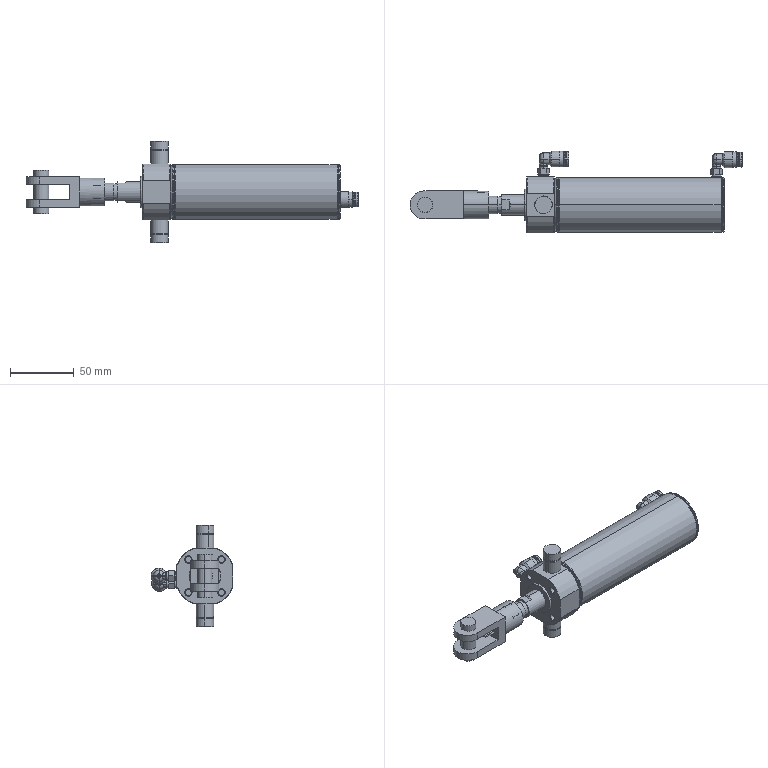Part | SolidWorks | features ReferencePattern 2, LocalLPattern 1 | 9 solids | 414 faces | box 261.082 x 64.35 x 80 mm | volume 157022 mm3 | cylinder 132 | cone 129 | plane 105 | spline 40 | torus 8 | commonest cylinder face diameters 14 x10 2.2 x8 4.917 x8 7.7 x8 11.6 x8 5.6 x6